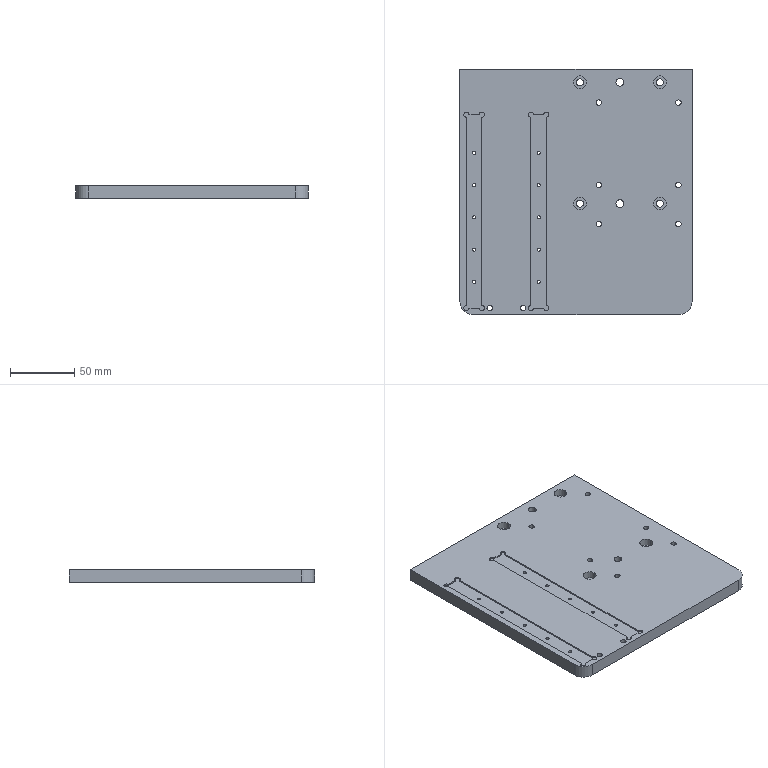Part | SolidWorks | features HoleWzd 6, ICE 2, Extrusion 1, Fillet 1, LPattern 1 | 1 solid | 98 faces | box 180 x 190 x 10 mm | volume 333166 mm3 | cylinder 74 | plane 20 | cone 4 | commonest cylinder face diameters 2.5 x20 4.2 x20 4 x12 5.5 x8 10 x8 6 x4